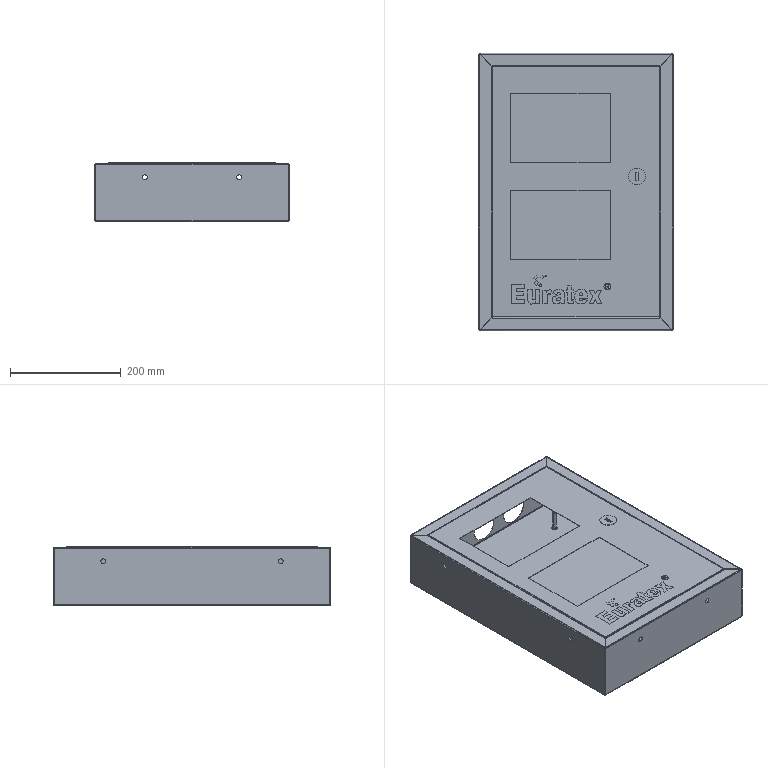Part | STEP file | 102000006842 | 16 solids | 351 faces | box 350 x 500 x 106.8 mm | volume 412738 mm3 | plane 225 | cylinder 70 | spline 48 | cone 8 | commonest cylinder face diameters 2 x16 3.6 x16 8.5 x12 6 x8 50 x6 2.279 x2